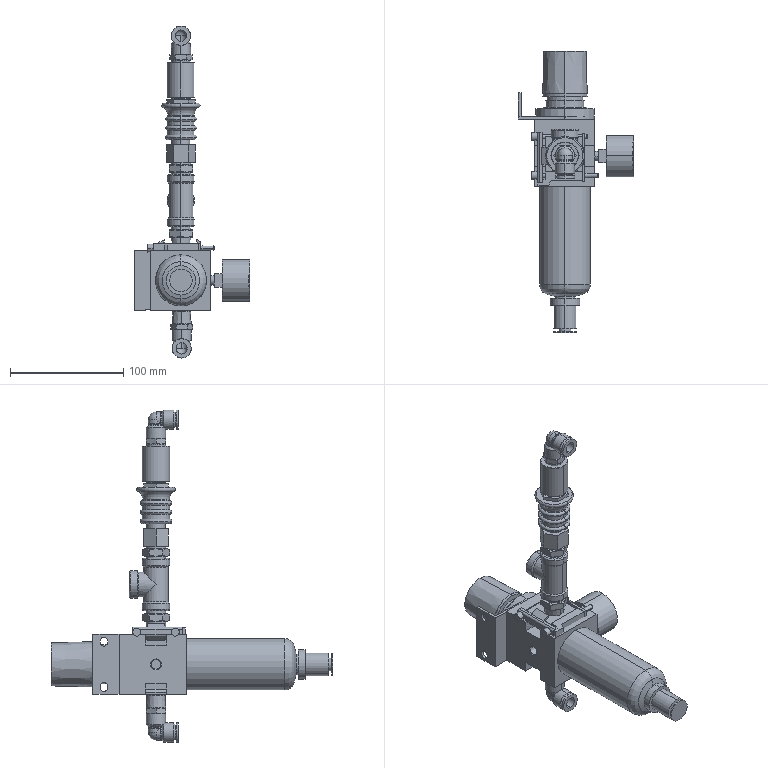Part | NX | 11 solids | 616 faces | box 101.5 x 248.5 x 292.94 mm | volume 498959 mm3 | plane 234 | cylinder 190 | cone 144 | torus 38 | spline 6 | sphere 4 | commonest cylinder face diameters 13.6 x24 16.8 x22 12.92 x16 17 x12 24 x12 4 x10